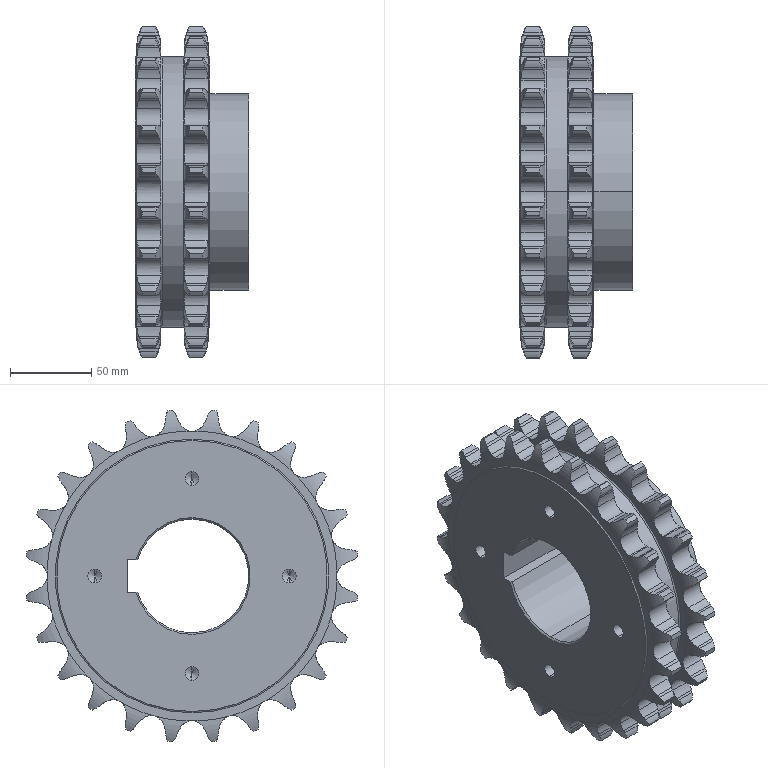Part | SolidWorks | features Revolution 3, Chamfer 2, Cut 2, ICE 2, CirPattern 1, HoleWzd 1, LPattern 1 | 1 solid | 557 faces | box 70 x 204.614 x 204.614 mm | volume 1174386 mm3 | cylinder 333 | plane 106 | torus 104 | cone 14 | commonest cylinder face diameters 22.999 x100 41.467 x100 16.059 x62 206 x48 8.5 x8 167 x6